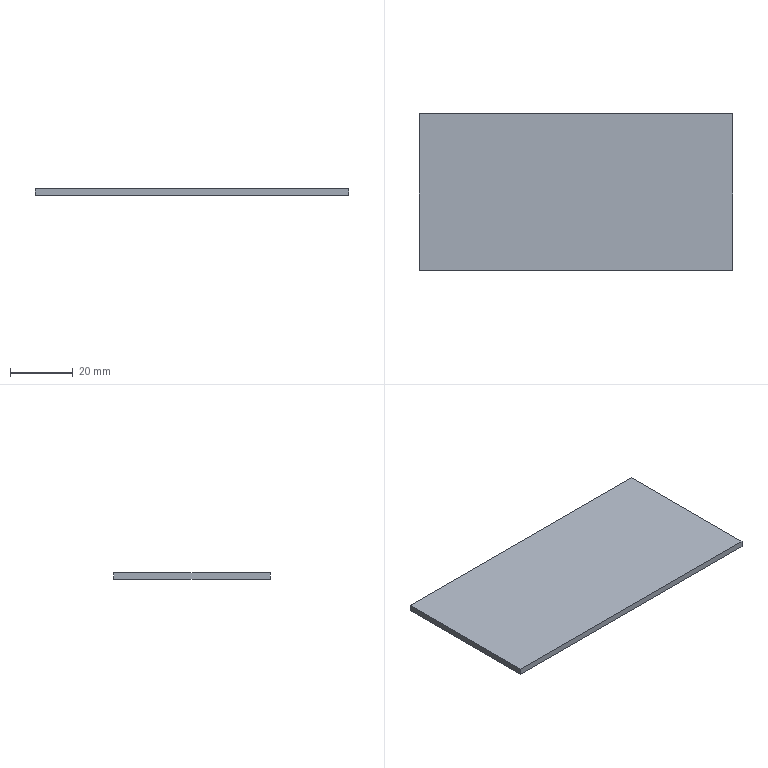Part | SolidWorks | features Extrusion 1 | 1 solid | 6 faces | box 100 x 50 x 2 mm | volume 10000 mm3 | plane 6
STEP:
#1=CARTESIAN_POINT('',(50.,-25.,0.));
#2=VERTEX_POINT('',#1);
#3=CARTESIAN_POINT('',(50.,25.,0.));
#4=VERTEX_POINT('',#3);
#5=CARTESIAN_POINT('',(50.,25.,0.));
#6=DIRECTION('',(0.,1.,0.));
#7=VECTOR('',#6,1000.);
#8=LINE('',#5,#7);
#9=EDGE_CURVE('',#2,#4,#8,.T.);
#10=ORIENTED_EDGE('',*,*,#9,.T.);
#11=CARTESIAN_POINT('',(50.,25.,2.));
#12=VERTEX_POINT('',#11);
#13=CARTESIAN_POINT('',(50.,25.,2.));
#14=DIRECTION('',(0.,0.,-1.));
#15=VECTOR('',#14,1000.);
#16=LINE('',#13,#15);
#17=EDGE_CURVE('',#12,#4,#16,.T.);
#18=ORIENTED_EDGE('',*,*,#17,.F.);
#19=CARTESIAN_POINT('',(50.,-25.,2.));
#20=VERTEX_POINT('',#19);
#21=CARTESIAN_POINT('',(50.,25.,2.));
#22=DIRECTION('',(0.,1.,0.));
#23=VECTOR('',#22,1000.);
#24=LINE('',#21,#23);
#25=EDGE_CURVE('',#20,#12,#24,.T.);
#26=ORIENTED_EDGE('',*,*,#25,.F.);
#27=CARTESIAN_POINT('',(50.,-25.,2.));
#28=DIRECTION('',(0.,0.,-1.));
#29=VECTOR('',#28,1000.);
#30=LINE('',#27,#29);
#31=EDGE_CURVE('',#20,#2,#30,.T.);
#32=ORIENTED_EDGE('',*,*,#31,.T.);
#33=EDGE_LOOP('',(#10,#18,#26,#32));
#34=FACE_OUTER_BOUND('',#33,.T.);
#35=CARTESIAN_POINT('',(50.,25.,2.));
#36=DIRECTION('',(-1.,0.,0.));
#37=DIRECTION('',(0.,-1.,0.));
#38=AXIS2_PLACEMENT_3D('',#35,#36,#37);
#39=PLANE('',#38);
#40=ADVANCED_FACE('',(#34),#39,.F.);
#41=CARTESIAN_POINT('',(-50.,25.,0.));
#42=VERTEX_POINT('',#41);
#43=CARTESIAN_POINT('',(-50.,25.,0.));
#44=DIRECTION('',(-1.,0.,0.));
#45=VECTOR('',#44,1000.);
#46=LINE('',#43,#45);
#47=EDGE_CURVE('',#4,#42,#46,.T.);
#48=ORIENTED_EDGE('',*,*,#47,.T.);
#49=CARTESIAN_POINT('',(-50.,25.,2.));
#50=VERTEX_POINT('',#49);
#51=CARTESIAN_POINT('',(-50.,25.,2.));
#52=DIRECTION('',(0.,0.,-1.));
#53=VECTOR('',#52,1000.);
#54=LINE('',#51,#53);
#55=EDGE_CURVE('',#50,#42,#54,.T.);
#56=ORIENTED_EDGE('',*,*,#55,.F.);
#57=CARTESIAN_POINT('',(-50.,25.,2.));
#58=DIRECTION('',(-1.,0.,0.));
#59=VECTOR('',#58,1000.);
#60=LINE('',#57,#59);
#61=EDGE_CURVE('',#12,#50,#60,.T.);
#62=ORIENTED_EDGE('',*,*,#61,.F.);
#63=ORIENTED_EDGE('',*,*,#17,.T.);
#64=EDGE_LOOP('',(#48,#56,#62,#63));
#65=FACE_OUTER_BOUND('',#64,.T.);
#66=CARTESIAN_POINT('',(-50.,25.,2.));
#67=DIRECTION('',(0.,-1.,0.));
#68=DIRECTION('',(0.,0.,-1.));
#69=AXIS2_PLACEMENT_3D('',#66,#67,#68);
#70=PLANE('',#69);
#71=ADVANCED_FACE('',(#65),#70,.F.);
#72=CARTESIAN_POINT('',(-50.,-25.,0.));
#73=VERTEX_POINT('',#72);
#74=CARTESIAN_POINT('',(-50.,25.,0.));
#75=DIRECTION('',(0.,-1.,0.));
#76=VECTOR('',#75,1000.);
#77=LINE('',#74,#76);
#78=EDGE_CURVE('',#42,#73,#77,.T.);
#79=ORIENTED_EDGE('',*,*,#78,.T.);
#80=CARTESIAN_POINT('',(-50.,-25.,2.));
#81=VERTEX_POINT('',#80);
#82=CARTESIAN_POINT('',(-50.,-25.,2.));
#83=DIRECTION('',(0.,0.,-1.));
#84=VECTOR('',#83,1000.);
#85=LINE('',#82,#84);
#86=EDGE_CURVE('',#81,#73,#85,.T.);
#87=ORIENTED_EDGE('',*,*,#86,.F.);
#88=CARTESIAN_POINT('',(-50.,25.,2.));
#89=DIRECTION('',(0.,-1.,0.));
#90=VECTOR('',#89,1000.);
#91=LINE('',#88,#90);
#92=EDGE_CURVE('',#50,#81,#91,.T.);
#93=ORIENTED_EDGE('',*,*,#92,.F.);
#94=ORIENTED_EDGE('',*,*,#55,.T.);
#95=EDGE_LOOP('',(#79,#87,#93,#94));
#96=FACE_OUTER_BOUND('',#95,.T.);
#97=CARTESIAN_POINT('',(-50.,25.,2.));
#98=DIRECTION('',(1.,0.,0.));
#99=DIRECTION('',(0.,1.,0.));
#100=AXIS2_PLACEMENT_3D('',#97,#98,#99);
#101=PLANE('',#100);
#102=ADVANCED_FACE('',(#96),#101,.F.);
#103=CARTESIAN_POINT('',(-50.,-25.,0.));
#104=DIRECTION('',(1.,0.,0.));
#105=VECTOR('',#104,1000.);
#106=LINE('',#103,#105);
#107=EDGE_CURVE('',#73,#2,#106,.T.);
#108=ORIENTED_EDGE('',*,*,#107,.T.);
#109=ORIENTED_EDGE('',*,*,#31,.F.);
#110=CARTESIAN_POINT('',(-50.,-25.,2.));
#111=DIRECTION('',(1.,0.,0.));
#112=VECTOR('',#111,1000.);
#113=LINE('',#110,#112);
#114=EDGE_CURVE('',#81,#20,#113,.T.);
#115=ORIENTED_EDGE('',*,*,#114,.F.);
#116=ORIENTED_EDGE('',*,*,#86,.T.);
#117=EDGE_LOOP('',(#108,#109,#115,#116));
#118=FACE_OUTER_BOUND('',#117,.T.);
#119=CARTESIAN_POINT('',(-50.,-25.,2.));
#120=DIRECTION('',(0.,1.,0.));
#121=DIRECTION('',(0.,0.,1.));
#122=AXIS2_PLACEMENT_3D('',#119,#120,#121);
#123=PLANE('',#122);
#124=ADVANCED_FACE('',(#118),#123,.F.);
#125=ORIENTED_EDGE('',*,*,#25,.T.);
#126=ORIENTED_EDGE('',*,*,#61,.T.);
#127=ORIENTED_EDGE('',*,*,#92,.T.);
#128=ORIENTED_EDGE('',*,*,#114,.T.);
#129=EDGE_LOOP('',(#125,#126,#127,#128));
#130=FACE_OUTER_BOUND('',#129,.T.);
#131=CARTESIAN_POINT('',(0.,0.,2.));
#132=DIRECTION('',(0.,0.,1.));
#133=DIRECTION('',(1.,0.,0.));
#134=AXIS2_PLACEMENT_3D('',#131,#132,#133);
#135=PLANE('',#134);
#136=ADVANCED_FACE('',(#130),#135,.T.);
#137=ORIENTED_EDGE('',*,*,#9,.F.);
#138=ORIENTED_EDGE('',*,*,#107,.F.);
#139=ORIENTED_EDGE('',*,*,#78,.F.);
#140=ORIENTED_EDGE('',*,*,#47,.F.);
#141=EDGE_LOOP('',(#137,#138,#139,#140));
#142=FACE_OUTER_BOUND('',#141,.T.);
#143=CARTESIAN_POINT('',(0.,0.,0.));
#144=DIRECTION('',(0.,0.,1.));
#145=DIRECTION('',(1.,0.,0.));
#146=AXIS2_PLACEMENT_3D('',#143,#144,#145);
#147=PLANE('',#146);
#148=ADVANCED_FACE('',(#142),#147,.F.);
#149=CLOSED_SHELL('',(#40,#71,#102,#124,#136,#148));
#150=MANIFOLD_SOLID_BREP('',#149);
#151=CARTESIAN_POINT('',(0.,0.,0.));
#152=DIRECTION('',(0.,0.,1.));
#153=DIRECTION('',(1.,0.,0.));
#154=AXIS2_PLACEMENT_3D('',#151,#152,#153);
#155=(LENGTH_UNIT()NAMED_UNIT(*)SI_UNIT(.MILLI.,.METRE.));
#156=UNCERTAINTY_MEASURE_WITH_UNIT(LENGTH_MEASURE(0.00001),#155,'','');
#157=(NAMED_UNIT(*)PLANE_ANGLE_UNIT()SI_UNIT($,.RADIAN.));
#158=(NAMED_UNIT(*)SI_UNIT($,.STERADIAN.)SOLID_ANGLE_UNIT());
#159=(GEOMETRIC_REPRESENTATION_CONTEXT(3)GLOBAL_UNCERTAINTY_ASSIGNED_CONTEXT((#156))GLOBAL_UNIT_ASSIGNED_CONTEXT((#155,#157,#158))REPRESENTATION_CONTEXT('',''));
#160=ADVANCED_BREP_SHAPE_REPRESENTATION('',(#150,#154),#159);